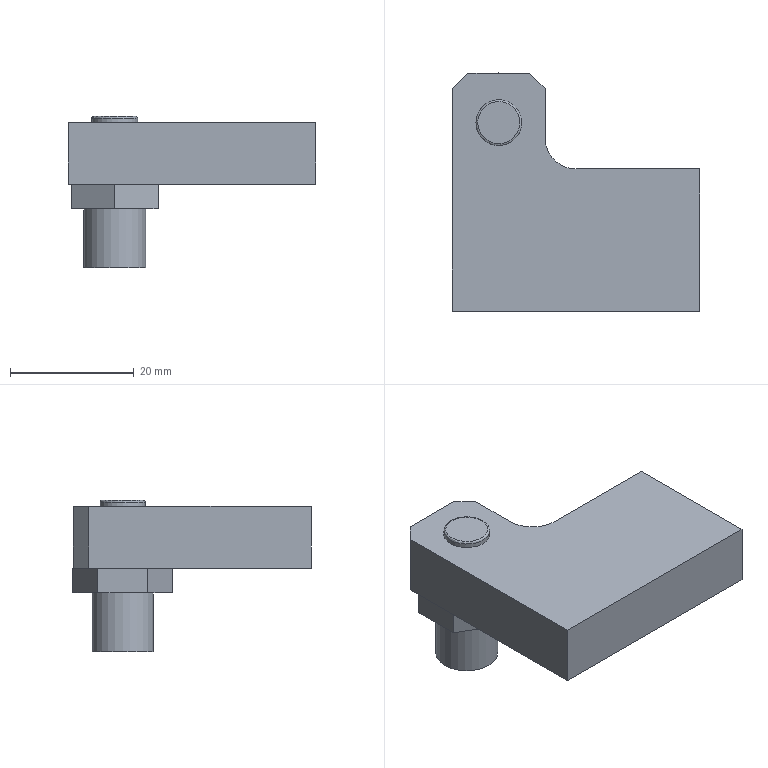Part | NX | 1 solid | 79 faces | box 40 x 38.584 x 24.5 mm | volume 12530 mm3 | plane 63 | cylinder 11 | cone 4 | spline 1 | commonest cylinder face diameters 8.5 x4 9 x4 10 x2 7.4 x1